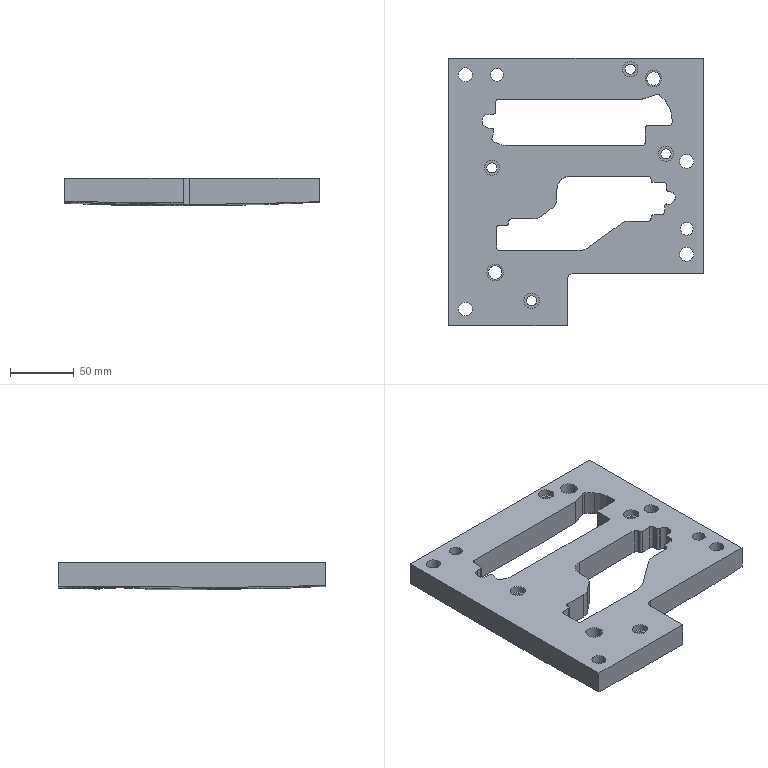Part | STEP file | 428_id666_x_t | 1 solid | 137 faces | box 200 x 210 x 21.719 mm | volume 522666 mm3 | cylinder 49 | plane 48 | spline 37 | other 3 | commonest cylinder face diameters 5 x12 12 x6 3 x5 11 x5 8 x4 17 x4